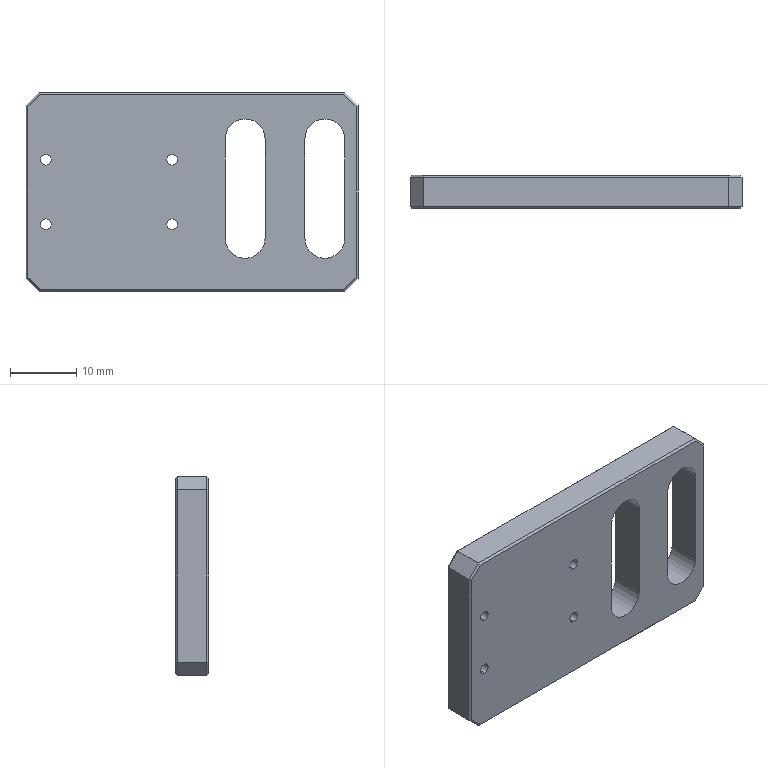Part | SolidWorks | features ICE 3, Chamfer 2, HoleWzd 2, CornerTrim 1, FlatPattern 1, SMBaseFlange 1, SheetMetal 1 | 1 solid | 44 faces | box 50 x 5 x 30 mm | volume 6223 mm3 | plane 30 | cylinder 14 | commonest cylinder face diameters 1.6 x8 6 x6
STEP:
#1=CARTESIAN_POINT('',(40.,0.,11.));
#2=VERTEX_POINT('',#1);
#3=CARTESIAN_POINT('',(43.,0.,8.));
#4=VERTEX_POINT('',#3);
#5=CARTESIAN_POINT('',(40.,0.,8.));
#6=DIRECTION('',(0.,1.,0.));
#7=DIRECTION('',(0.,0.,1.));
#8=AXIS2_PLACEMENT_3D('',#5,#6,#7);
#9=CIRCLE('',#8,3.);
#10=EDGE_CURVE('',#2,#4,#9,.T.);
#11=ORIENTED_EDGE('',*,*,#10,.F.);
#12=CARTESIAN_POINT('',(40.,5.,11.));
#13=VERTEX_POINT('',#12);
#14=CARTESIAN_POINT('',(40.,0.,11.));
#15=DIRECTION('',(0.,1.,0.));
#16=VECTOR('',#15,1000.);
#17=LINE('',#14,#16);
#18=EDGE_CURVE('',#2,#13,#17,.T.);
#19=ORIENTED_EDGE('',*,*,#18,.T.);
#20=CARTESIAN_POINT('',(43.,5.,8.));
#21=VERTEX_POINT('',#20);
#22=CARTESIAN_POINT('',(40.,5.,8.));
#23=DIRECTION('',(0.,1.,0.));
#24=DIRECTION('',(0.,0.,1.));
#25=AXIS2_PLACEMENT_3D('',#22,#23,#24);
#26=CIRCLE('',#25,3.);
#27=EDGE_CURVE('',#13,#21,#26,.T.);
#28=ORIENTED_EDGE('',*,*,#27,.T.);
#29=CARTESIAN_POINT('',(43.,0.,8.));
#30=DIRECTION('',(0.,1.,0.));
#31=VECTOR('',#30,1000.);
#32=LINE('',#29,#31);
#33=EDGE_CURVE('',#4,#21,#32,.T.);
#34=ORIENTED_EDGE('',*,*,#33,.F.);
#35=EDGE_LOOP('',(#11,#19,#28,#34));
#36=FACE_OUTER_BOUND('',#35,.T.);
#37=CARTESIAN_POINT('',(40.,0.,8.));
#38=DIRECTION('',(0.,1.,0.));
#39=DIRECTION('',(0.,0.,1.));
#40=AXIS2_PLACEMENT_3D('',#37,#38,#39);
#41=CYLINDRICAL_SURFACE('',#40,3.);
#42=ADVANCED_FACE('',(#36),#41,.F.);
#43=CARTESIAN_POINT('',(28.,0.,11.));
#44=VERTEX_POINT('',#43);
#45=CARTESIAN_POINT('',(31.,0.,8.));
#46=VERTEX_POINT('',#45);
#47=CARTESIAN_POINT('',(28.,0.,8.));
#48=DIRECTION('',(0.,1.,0.));
#49=DIRECTION('',(0.,0.,1.));
#50=AXIS2_PLACEMENT_3D('',#47,#48,#49);
#51=CIRCLE('',#50,3.);
#52=EDGE_CURVE('',#44,#46,#51,.T.);
#53=ORIENTED_EDGE('',*,*,#52,.F.);
#54=CARTESIAN_POINT('',(28.,5.,11.));
#55=VERTEX_POINT('',#54);
#56=CARTESIAN_POINT('',(28.,0.,11.));
#57=DIRECTION('',(0.,1.,0.));
#58=VECTOR('',#57,1000.);
#59=LINE('',#56,#58);
#60=EDGE_CURVE('',#44,#55,#59,.T.);
#61=ORIENTED_EDGE('',*,*,#60,.T.);
#62=CARTESIAN_POINT('',(31.,5.,8.));
#63=VERTEX_POINT('',#62);
#64=CARTESIAN_POINT('',(28.,5.,8.));
#65=DIRECTION('',(0.,1.,0.));
#66=DIRECTION('',(0.,0.,1.));
#67=AXIS2_PLACEMENT_3D('',#64,#65,#66);
#68=CIRCLE('',#67,3.);
#69=EDGE_CURVE('',#55,#63,#68,.T.);
#70=ORIENTED_EDGE('',*,*,#69,.T.);
#71=CARTESIAN_POINT('',(31.,0.,8.));
#72=DIRECTION('',(0.,1.,0.));
#73=VECTOR('',#72,1000.);
#74=LINE('',#71,#73);
#75=EDGE_CURVE('',#46,#63,#74,.T.);
#76=ORIENTED_EDGE('',*,*,#75,.F.);
#77=EDGE_LOOP('',(#53,#61,#70,#76));
#78=FACE_OUTER_BOUND('',#77,.T.);
#79=CARTESIAN_POINT('',(28.,0.,8.));
#80=DIRECTION('',(0.,1.,0.));
#81=DIRECTION('',(0.,0.,1.));
#82=AXIS2_PLACEMENT_3D('',#79,#80,#81);
#83=CYLINDRICAL_SURFACE('',#82,3.);
#84=ADVANCED_FACE('',(#78),#83,.F.);
#85=CARTESIAN_POINT('',(17.,0.,-5.65));
#86=VERTEX_POINT('',#85);
#87=CARTESIAN_POINT('',(17.,0.,-4.05));
#88=VERTEX_POINT('',#87);
#89=CARTESIAN_POINT('',(17.,0.,-4.85));
#90=DIRECTION('',(0.,1.,0.));
#91=DIRECTION('',(0.,0.,1.));
#92=AXIS2_PLACEMENT_3D('',#89,#90,#91);
#93=CIRCLE('',#92,0.8);
#94=EDGE_CURVE('',#86,#88,#93,.T.);
#95=ORIENTED_EDGE('',*,*,#94,.F.);
#96=CARTESIAN_POINT('',(17.,5.,-5.65));
#97=VERTEX_POINT('',#96);
#98=CARTESIAN_POINT('',(17.,5.,-5.65));
#99=DIRECTION('',(0.,1.,0.));
#100=VECTOR('',#99,1000.);
#101=LINE('',#98,#100);
#102=EDGE_CURVE('',#86,#97,#101,.T.);
#103=ORIENTED_EDGE('',*,*,#102,.T.);
#104=CARTESIAN_POINT('',(17.,5.,-4.05));
#105=VERTEX_POINT('',#104);
#106=CARTESIAN_POINT('',(17.,5.,-4.85));
#107=DIRECTION('',(0.,1.,0.));
#108=DIRECTION('',(0.,0.,1.));
#109=AXIS2_PLACEMENT_3D('',#106,#107,#108);
#110=CIRCLE('',#109,0.8);
#111=EDGE_CURVE('',#97,#105,#110,.T.);
#112=ORIENTED_EDGE('',*,*,#111,.T.);
#113=CARTESIAN_POINT('',(17.,5.,-4.05));
#114=DIRECTION('',(0.,1.,0.));
#115=VECTOR('',#114,1000.);
#116=LINE('',#113,#115);
#117=EDGE_CURVE('',#88,#105,#116,.T.);
#118=ORIENTED_EDGE('',*,*,#117,.F.);
#119=EDGE_LOOP('',(#95,#103,#112,#118));
#120=FACE_OUTER_BOUND('',#119,.T.);
#121=CARTESIAN_POINT('',(17.,5.,-4.85));
#122=DIRECTION('',(0.,1.,0.));
#123=DIRECTION('',(0.,0.,1.));
#124=AXIS2_PLACEMENT_3D('',#121,#122,#123);
#125=CYLINDRICAL_SURFACE('',#124,0.8);
#126=ADVANCED_FACE('',(#120),#125,.F.);
#127=CARTESIAN_POINT('',(-2.,0.,4.05));
#128=VERTEX_POINT('',#127);
#129=CARTESIAN_POINT('',(-2.,0.,5.65));
#130=VERTEX_POINT('',#129);
#131=CARTESIAN_POINT('',(-2.,0.,4.85));
#132=DIRECTION('',(0.,1.,0.));
#133=DIRECTION('',(0.,0.,1.));
#134=AXIS2_PLACEMENT_3D('',#131,#132,#133);
#135=CIRCLE('',#134,0.8);
#136=EDGE_CURVE('',#128,#130,#135,.T.);
#137=ORIENTED_EDGE('',*,*,#136,.F.);
#138=CARTESIAN_POINT('',(-2.,5.,4.05));
#139=VERTEX_POINT('',#138);
#140=CARTESIAN_POINT('',(-2.,5.,4.05));
#141=DIRECTION('',(0.,1.,0.));
#142=VECTOR('',#141,1000.);
#143=LINE('',#140,#142);
#144=EDGE_CURVE('',#128,#139,#143,.T.);
#145=ORIENTED_EDGE('',*,*,#144,.T.);
#146=CARTESIAN_POINT('',(-2.,5.,5.65));
#147=VERTEX_POINT('',#146);
#148=CARTESIAN_POINT('',(-2.,5.,4.85));
#149=DIRECTION('',(0.,1.,0.));
#150=DIRECTION('',(0.,0.,1.));
#151=AXIS2_PLACEMENT_3D('',#148,#149,#150);
#152=CIRCLE('',#151,0.8);
#153=EDGE_CURVE('',#139,#147,#152,.T.);
#154=ORIENTED_EDGE('',*,*,#153,.T.);
#155=CARTESIAN_POINT('',(-2.,5.,5.65));
#156=DIRECTION('',(0.,1.,0.));
#157=VECTOR('',#156,1000.);
#158=LINE('',#155,#157);
#159=EDGE_CURVE('',#130,#147,#158,.T.);
#160=ORIENTED_EDGE('',*,*,#159,.F.);
#161=EDGE_LOOP('',(#137,#145,#154,#160));
#162=FACE_OUTER_BOUND('',#161,.T.);
#163=CARTESIAN_POINT('',(-2.,5.,4.85));
#164=DIRECTION('',(0.,1.,0.));
#165=DIRECTION('',(0.,0.,1.));
#166=AXIS2_PLACEMENT_3D('',#163,#164,#165);
#167=CYLINDRICAL_SURFACE('',#166,0.8);
#168=ADVANCED_FACE('',(#162),#167,.F.);
#169=CARTESIAN_POINT('',(-2.,0.,-5.65));
#170=VERTEX_POINT('',#169);
#171=CARTESIAN_POINT('',(-2.,0.,-4.05));
#172=VERTEX_POINT('',#171);
#173=CARTESIAN_POINT('',(-2.,0.,-4.85));
#174=DIRECTION('',(0.,1.,0.));
#175=DIRECTION('',(0.,0.,1.));
#176=AXIS2_PLACEMENT_3D('',#173,#174,#175);
#177=CIRCLE('',#176,0.8);
#178=EDGE_CURVE('',#170,#172,#177,.T.);
#179=ORIENTED_EDGE('',*,*,#178,.F.);
#180=CARTESIAN_POINT('',(-2.,5.,-5.65));
#181=VERTEX_POINT('',#180);
#182=CARTESIAN_POINT('',(-2.,5.,-5.65));
#183=DIRECTION('',(0.,1.,0.));
#184=VECTOR('',#183,1000.);
#185=LINE('',#182,#184);
#186=EDGE_CURVE('',#170,#181,#185,.T.);
#187=ORIENTED_EDGE('',*,*,#186,.T.);
#188=CARTESIAN_POINT('',(-2.,5.,-4.05));
#189=VERTEX_POINT('',#188);
#190=CARTESIAN_POINT('',(-2.,5.,-4.85));
#191=DIRECTION('',(0.,1.,0.));
#192=DIRECTION('',(0.,0.,1.));
#193=AXIS2_PLACEMENT_3D('',#190,#191,#192);
#194=CIRCLE('',#193,0.8);
#195=EDGE_CURVE('',#181,#189,#194,.T.);
#196=ORIENTED_EDGE('',*,*,#195,.T.);
#197=CARTESIAN_POINT('',(-2.,5.,-4.05));
#198=DIRECTION('',(0.,1.,0.));
#199=VECTOR('',#198,1000.);
#200=LINE('',#197,#199);
#201=EDGE_CURVE('',#172,#189,#200,.T.);
#202=ORIENTED_EDGE('',*,*,#201,.F.);
#203=EDGE_LOOP('',(#179,#187,#196,#202));
#204=FACE_OUTER_BOUND('',#203,.T.);
#205=CARTESIAN_POINT('',(-2.,5.,-4.85));
#206=DIRECTION('',(0.,1.,0.));
#207=DIRECTION('',(0.,0.,1.));
#208=AXIS2_PLACEMENT_3D('',#205,#206,#207);
#209=CYLINDRICAL_SURFACE('',#208,0.8);
#210=ADVANCED_FACE('',(#204),#209,.F.);
#211=CARTESIAN_POINT('',(17.,0.,4.05));
#212=VERTEX_POINT('',#211);
#213=CARTESIAN_POINT('',(17.,0.,5.65));
#214=VERTEX_POINT('',#213);
#215=CARTESIAN_POINT('',(17.,0.,4.85));
#216=DIRECTION('',(0.,1.,0.));
#217=DIRECTION('',(0.,0.,1.));
#218=AXIS2_PLACEMENT_3D('',#215,#216,#217);
#219=CIRCLE('',#218,0.8);
#220=EDGE_CURVE('',#212,#214,#219,.T.);
#221=ORIENTED_EDGE('',*,*,#220,.F.);
#222=CARTESIAN_POINT('',(17.,5.,4.05));
#223=VERTEX_POINT('',#222);
#224=CARTESIAN_POINT('',(17.,5.,4.05));
#225=DIRECTION('',(0.,1.,0.));
#226=VECTOR('',#225,1000.);
#227=LINE('',#224,#226);
#228=EDGE_CURVE('',#212,#223,#227,.T.);
#229=ORIENTED_EDGE('',*,*,#228,.T.);
#230=CARTESIAN_POINT('',(17.,5.,5.65));
#231=VERTEX_POINT('',#230);
#232=CARTESIAN_POINT('',(17.,5.,4.85));
#233=DIRECTION('',(0.,1.,0.));
#234=DIRECTION('',(0.,0.,1.));
#235=AXIS2_PLACEMENT_3D('',#232,#233,#234);
#236=CIRCLE('',#235,0.8);
#237=EDGE_CURVE('',#223,#231,#236,.T.);
#238=ORIENTED_EDGE('',*,*,#237,.T.);
#239=CARTESIAN_POINT('',(17.,5.,5.65));
#240=DIRECTION('',(0.,1.,0.));
#241=VECTOR('',#240,1000.);
#242=LINE('',#239,#241);
#243=EDGE_CURVE('',#214,#231,#242,.T.);
#244=ORIENTED_EDGE('',*,*,#243,.F.);
#245=EDGE_LOOP('',(#221,#229,#238,#244));
#246=FACE_OUTER_BOUND('',#245,.T.);
#247=CARTESIAN_POINT('',(17.,5.,4.85));
#248=DIRECTION('',(0.,1.,0.));
#249=DIRECTION('',(0.,0.,1.));
#250=AXIS2_PLACEMENT_3D('',#247,#248,#249);
#251=CYLINDRICAL_SURFACE('',#250,0.8);
#252=ADVANCED_FACE('',(#246),#251,.F.);
#253=CARTESIAN_POINT('',(43.,4.7,-15.));
#254=VERTEX_POINT('',#253);
#255=CARTESIAN_POINT('',(43.,0.3,-15.));
#256=VERTEX_POINT('',#255);
#257=CARTESIAN_POINT('',(43.,5.5,-15.));
#258=DIRECTION('',(0.,-1.,0.));
#259=VECTOR('',#258,1000.);
#260=LINE('',#257,#259);
#261=EDGE_CURVE('',#254,#256,#260,.T.);
#262=ORIENTED_EDGE('',*,*,#261,.T.);
#263=CARTESIAN_POINT('',(-3.,0.3,-15.));
#264=VERTEX_POINT('',#263);
#265=CARTESIAN_POINT('',(-40.,0.3,-15.));
#266=DIRECTION('',(-1.,0.,0.));
#267=VECTOR('',#266,1000.);
#268=LINE('',#265,#267);
#269=EDGE_CURVE('',#256,#264,#268,.T.);
#270=ORIENTED_EDGE('',*,*,#269,.T.);
#271=CARTESIAN_POINT('',(-3.,4.7,-15.));
#272=VERTEX_POINT('',#271);
#273=CARTESIAN_POINT('',(-3.,5.,-15.));
#274=DIRECTION('',(0.,1.,0.));
#275=VECTOR('',#274,1000.);
#276=LINE('',#273,#275);
#277=EDGE_CURVE('',#264,#272,#276,.T.);
#278=ORIENTED_EDGE('',*,*,#277,.T.);
#279=CARTESIAN_POINT('',(43.,4.7,-15.));
#280=DIRECTION('',(1.,0.,0.));
#281=VECTOR('',#280,1000.);
#282=LINE('',#279,#281);
#283=EDGE_CURVE('',#272,#254,#282,.T.);
#284=ORIENTED_EDGE('',*,*,#283,.T.);
#285=EDGE_LOOP('',(#262,#270,#278,#284));
#286=FACE_OUTER_BOUND('',#285,.T.);
#287=CARTESIAN_POINT('',(-40.,5.5,-15.));
#288=DIRECTION('',(0.,0.,-1.));
#289=DIRECTION('',(-1.,0.,0.));
#290=AXIS2_PLACEMENT_3D('',#287,#288,#289);
#291=PLANE('',#290);
#292=ADVANCED_FACE('',(#286),#291,.T.);
#293=CARTESIAN_POINT('',(43.,0.,-7.));
#294=VERTEX_POINT('',#293);
#295=CARTESIAN_POINT('',(37.,0.,-7.));
#296=VERTEX_POINT('',#295);
#297=CARTESIAN_POINT('',(40.,0.,-7.));
#298=DIRECTION('',(0.,1.,0.));
#299=DIRECTION('',(0.,0.,1.));
#300=AXIS2_PLACEMENT_3D('',#297,#298,#299);
#301=CIRCLE('',#300,3.);
#302=EDGE_CURVE('',#294,#296,#301,.T.);
#303=ORIENTED_EDGE('',*,*,#302,.T.);
#304=CARTESIAN_POINT('',(37.,0.,8.));
#305=VERTEX_POINT('',#304);
#306=CARTESIAN_POINT('',(37.,0.,-7.));
#307=DIRECTION('',(0.,0.,1.));
#308=VECTOR('',#307,1000.);
#309=LINE('',#306,#308);
#310=EDGE_CURVE('',#296,#305,#309,.T.);
#311=ORIENTED_EDGE('',*,*,#310,.T.);
#312=CARTESIAN_POINT('',(40.,0.,8.));
#313=DIRECTION('',(0.,1.,0.));
#314=DIRECTION('',(0.,0.,1.));
#315=AXIS2_PLACEMENT_3D('',#312,#313,#314);
#316=CIRCLE('',#315,3.);
#317=EDGE_CURVE('',#305,#2,#316,.T.);
#318=ORIENTED_EDGE('',*,*,#317,.T.);
#319=ORIENTED_EDGE('',*,*,#10,.T.);
#320=CARTESIAN_POINT('',(43.,0.,-7.));
#321=DIRECTION('',(0.,0.,-1.));
#322=VECTOR('',#321,1000.);
#323=LINE('',#320,#322);
#324=EDGE_CURVE('',#4,#294,#323,.T.);
#325=ORIENTED_EDGE('',*,*,#324,.T.);
#326=EDGE_LOOP('',(#303,#311,#318,#319,#325));
#327=FACE_BOUND('',#326,.T.);
#328=CARTESIAN_POINT('',(31.,0.,-7.));
#329=VERTEX_POINT('',#328);
#330=CARTESIAN_POINT('',(25.,0.,-7.));
#331=VERTEX_POINT('',#330);
#332=CARTESIAN_POINT('',(28.,0.,-7.));
#333=DIRECTION('',(0.,1.,0.));
#334=DIRECTION('',(0.,0.,1.));
#335=AXIS2_PLACEMENT_3D('',#332,#333,#334);
#336=CIRCLE('',#335,3.);
#337=EDGE_CURVE('',#329,#331,#336,.T.);
#338=ORIENTED_EDGE('',*,*,#337,.T.);
#339=CARTESIAN_POINT('',(25.,0.,8.));
#340=VERTEX_POINT('',#339);
#341=CARTESIAN_POINT('',(25.,0.,-7.));
#342=DIRECTION('',(0.,0.,1.));
#343=VECTOR('',#342,1000.);
#344=LINE('',#341,#343);
#345=EDGE_CURVE('',#331,#340,#344,.T.);
#346=ORIENTED_EDGE('',*,*,#345,.T.);
#347=CARTESIAN_POINT('',(28.,0.,8.));
#348=DIRECTION('',(0.,1.,0.));
#349=DIRECTION('',(0.,0.,1.));
#350=AXIS2_PLACEMENT_3D('',#347,#348,#349);
#351=CIRCLE('',#350,3.);
#352=EDGE_CURVE('',#340,#44,#351,.T.);
#353=ORIENTED_EDGE('',*,*,#352,.T.);
#354=ORIENTED_EDGE('',*,*,#52,.T.);
#355=CARTESIAN_POINT('',(31.,0.,-7.));
#356=DIRECTION('',(0.,0.,-1.));
#357=VECTOR('',#356,1000.);
#358=LINE('',#355,#357);
#359=EDGE_CURVE('',#46,#329,#358,.T.);
#360=ORIENTED_EDGE('',*,*,#359,.T.);
#361=EDGE_LOOP('',(#338,#346,#353,#354,#360));
#362=FACE_BOUND('',#361,.T.);
#363=CARTESIAN_POINT('',(-4.7,0.,12.876));
#364=VERTEX_POINT('',#363);
#365=CARTESIAN_POINT('',(-4.7,0.,-12.876));
#366=VERTEX_POINT('',#365);
#367=CARTESIAN_POINT('',(-4.7,0.,-13.));
#368=DIRECTION('',(0.,0.,-1.));
#369=VECTOR('',#368,1000.);
#370=LINE('',#367,#369);
#371=EDGE_CURVE('',#364,#366,#370,.T.);
#372=ORIENTED_EDGE('',*,*,#371,.T.);
#373=CARTESIAN_POINT('',(-2.876,0.,-14.7));
#374=VERTEX_POINT('',#373);
#375=CARTESIAN_POINT('',(-38.788,0.,21.212));
#376=DIRECTION('',(0.7071,0.,-0.7071));
#377=VECTOR('',#376,1000.);
#378=LINE('',#375,#377);
#379=EDGE_CURVE('',#366,#374,#378,.T.);
#380=ORIENTED_EDGE('',*,*,#379,.T.);
#381=CARTESIAN_POINT('',(42.876,0.,-14.7));
#382=VERTEX_POINT('',#381);
#383=CARTESIAN_POINT('',(-45.,0.,-14.7));
#384=DIRECTION('',(1.,0.,0.));
#385=VECTOR('',#384,1000.);
#386=LINE('',#383,#385);
#387=EDGE_CURVE('',#374,#382,#386,.T.);
#388=ORIENTED_EDGE('',*,*,#387,.T.);
#389=CARTESIAN_POINT('',(44.7,0.,-12.876));
#390=VERTEX_POINT('',#389);
#391=CARTESIAN_POINT('',(13.788,0.,-43.788));
#392=DIRECTION('',(0.7071,0.,0.7071));
#393=VECTOR('',#392,1000.);
#394=LINE('',#391,#393);
#395=EDGE_CURVE('',#382,#390,#394,.T.);
#396=ORIENTED_EDGE('',*,*,#395,.T.);
#397=CARTESIAN_POINT('',(44.7,0.,12.876));
#398=VERTEX_POINT('',#397);
#399=CARTESIAN_POINT('',(44.7,0.,15.));
#400=DIRECTION('',(0.,0.,1.));
#401=VECTOR('',#400,1000.);
#402=LINE('',#399,#401);
#403=EDGE_CURVE('',#390,#398,#402,.T.);
#404=ORIENTED_EDGE('',*,*,#403,.T.);
#405=CARTESIAN_POINT('',(42.876,0.,14.7));
#406=VERTEX_POINT('',#405);
#407=CARTESIAN_POINT('',(-1.212,0.,58.788));
#408=DIRECTION('',(-0.7071,0.,0.7071));
#409=VECTOR('',#408,1000.);
#410=LINE('',#407,#409);
#411=EDGE_CURVE('',#398,#406,#410,.T.);
#412=ORIENTED_EDGE('',*,*,#411,.T.);
#413=CARTESIAN_POINT('',(-2.876,0.,14.7));
#414=VERTEX_POINT('',#413);
#415=CARTESIAN_POINT('',(-45.,0.,14.7));
#416=DIRECTION('',(-1.,0.,0.));
#417=VECTOR('',#416,1000.);
#418=LINE('',#415,#417);
#419=EDGE_CURVE('',#406,#414,#418,.T.);
#420=ORIENTED_EDGE('',*,*,#419,.T.);
#421=CARTESIAN_POINT('',(-23.788,0.,-6.212));
#422=DIRECTION('',(-0.7071,0.,-0.7071));
#423=VECTOR('',#422,1000.);
#424=LINE('',#421,#423);
#425=EDGE_CURVE('',#414,#364,#424,.T.);
#426=ORIENTED_EDGE('',*,*,#425,.T.);
#427=EDGE_LOOP('',(#372,#380,#388,#396,#404,#412,#420,#426));
#428=FACE_OUTER_BOUND('',#427,.T.);
#429=CARTESIAN_POINT('',(17.,0.,-4.85));
#430=DIRECTION('',(0.,1.,0.));
#431=DIRECTION('',(0.,0.,1.));
#432=AXIS2_PLACEMENT_3D('',#429,#430,#431);
#433=CIRCLE('',#432,0.8);
#434=EDGE_CURVE('',#88,#86,#433,.T.);
#435=ORIENTED_EDGE('',*,*,#434,.T.);
#436=ORIENTED_EDGE('',*,*,#94,.T.);
#437=EDGE_LOOP('',(#435,#436));
#438=FACE_BOUND('',#437,.T.);
#439=CARTESIAN_POINT('',(-2.,0.,4.85));
#440=DIRECTION('',(0.,1.,0.));
#441=DIRECTION('',(0.,0.,1.));
#442=AXIS2_PLACEMENT_3D('',#439,#440,#441);
#443=CIRCLE('',#442,0.8);
#444=EDGE_CURVE('',#130,#128,#443,.T.);
#445=ORIENTED_EDGE('',*,*,#444,.T.);
#446=ORIENTED_EDGE('',*,*,#136,.T.);
#447=EDGE_LOOP('',(#445,#446));
#448=FACE_BOUND('',#447,.T.);
#449=CARTESIAN_POINT('',(-2.,0.,-4.85));
#450=DIRECTION('',(0.,1.,0.));
#451=DIRECTION('',(0.,0.,1.));
#452=AXIS2_PLACEMENT_3D('',#449,#450,#451);
#453=CIRCLE('',#452,0.8);
#454=EDGE_CURVE('',#172,#170,#453,.T.);
#455=ORIENTED_EDGE('',*,*,#454,.T.);
#456=ORIENTED_EDGE('',*,*,#178,.T.);
#457=EDGE_LOOP('',(#455,#456));
#458=FACE_BOUND('',#457,.T.);
#459=CARTESIAN_POINT('',(17.,0.,4.85));
#460=DIRECTION('',(0.,1.,0.));
#461=DIRECTION('',(0.,0.,1.));
#462=AXIS2_PLACEMENT_3D('',#459,#460,#461);
#463=CIRCLE('',#462,0.8);
#464=EDGE_CURVE('',#214,#212,#463,.T.);
#465=ORIENTED_EDGE('',*,*,#464,.T.);
#466=ORIENTED_EDGE('',*,*,#220,.T.);
#467=EDGE_LOOP('',(#465,#466));
#468=FACE_BOUND('',#467,.T.);
#469=CARTESIAN_POINT('',(-45.,0.,15.));
#470=DIRECTION('',(0.,-1.,0.));
#471=DIRECTION('',(0.,0.,-1.));
#472=AXIS2_PLACEMENT_3D('',#469,#470,#471);
#473=PLANE('',#472);
#474=ADVANCED_FACE('',(#327,#362,#428,#438,#448,#458,#468),#473,.T.);
#475=CARTESIAN_POINT('',(45.,4.7,13.));
#476=VERTEX_POINT('',#475);
#477=CARTESIAN_POINT('',(45.,0.3,13.));
#478=VERTEX_POINT('',#477);
#479=CARTESIAN_POINT('',(45.,5.,13.));
#480=DIRECTION('',(0.,-1.,0.));
#481=VECTOR('',#480,1000.);
#482=LINE('',#479,#481);
#483=EDGE_CURVE('',#476,#478,#482,.T.);
#484=ORIENTED_EDGE('',*,*,#483,.T.);
#485=CARTESIAN_POINT('',(45.,0.3,-13.));
#486=VERTEX_POINT('',#485);
#487=CARTESIAN_POINT('',(45.,0.3,15.));
#488=DIRECTION('',(0.,0.,-1.));
#489=VECTOR('',#488,1000.);
#490=LINE('',#487,#489);
#491=EDGE_CURVE('',#478,#486,#490,.T.);
#492=ORIENTED_EDGE('',*,*,#491,.T.);
#493=CARTESIAN_POINT('',(45.,4.7,-13.));
#494=VERTEX_POINT('',#493);
#495=CARTESIAN_POINT('',(45.,5.,-13.));
#496=DIRECTION('',(0.,1.,0.));
#497=VECTOR('',#496,1000.);
#498=LINE('',#495,#497);
#499=EDGE_CURVE('',#486,#494,#498,.T.);
#500=ORIENTED_EDGE('',*,*,#499,.T.);
#501=CARTESIAN_POINT('',(45.,4.7,13.));
#502=DIRECTION('',(0.,0.,1.));
#503=VECTOR('',#502,1000.);
#504=LINE('',#501,#503);
#505=EDGE_CURVE('',#494,#476,#504,.T.);
#506=ORIENTED_EDGE('',*,*,#505,.T.);
#507=EDGE_LOOP('',(#484,#492,#500,#506));
#508=FACE_OUTER_BOUND('',#507,.T.);
#509=CARTESIAN_POINT('',(45.,5.,15.));
#510=DIRECTION('',(1.,0.,0.));
#511=DIRECTION('',(0.,0.,-1.));
#512=AXIS2_PLACEMENT_3D('',#509,#510,#511);
#513=PLANE('',#512);
#514=ADVANCED_FACE('',(#508),#513,.T.);
#515=CARTESIAN_POINT('',(44.7,5.,12.876));
#516=VERTEX_POINT('',#515);
#517=CARTESIAN_POINT('',(44.7,5.,-12.876));
#518=VERTEX_POINT('',#517);
#519=CARTESIAN_POINT('',(44.7,5.,-13.));
#520=DIRECTION('',(0.,0.,-1.));
#521=VECTOR('',#520,1000.);
#522=LINE('',#519,#521);
#523=EDGE_CURVE('',#516,#518,#522,.T.);
#524=ORIENTED_EDGE('',*,*,#523,.T.);
#525=CARTESIAN_POINT('',(42.876,5.,-14.7));
#526=VERTEX_POINT('',#525);
#527=CARTESIAN_POINT('',(42.788,5.,-14.788));
#528=DIRECTION('',(-0.7071,0.,-0.7071));
#529=VECTOR('',#528,1000.);
#530=LINE('',#527,#529);
#531=EDGE_CURVE('',#518,#526,#530,.T.);
#532=ORIENTED_EDGE('',*,*,#531,.T.);
#533=CARTESIAN_POINT('',(-2.876,5.,-14.7));
#534=VERTEX_POINT('',#533);
#535=CARTESIAN_POINT('',(-3.,5.,-14.7));
#536=DIRECTION('',(-1.,0.,0.));
#537=VECTOR('',#536,1000.);
#538=LINE('',#535,#537);
#539=EDGE_CURVE('',#526,#534,#538,.T.);
#540=ORIENTED_EDGE('',*,*,#539,.T.);
#541=CARTESIAN_POINT('',(-4.7,5.,-12.876));
#542=VERTEX_POINT('',#541);
#543=CARTESIAN_POINT('',(-4.788,5.,-12.788));
#544=DIRECTION('',(-0.7071,0.,0.7071));
#545=VECTOR('',#544,1000.);
#546=LINE('',#543,#545);
#547=EDGE_CURVE('',#534,#542,#546,.T.);
#548=ORIENTED_EDGE('',*,*,#547,.T.);
#549=CARTESIAN_POINT('',(-4.7,5.,12.876));
#550=VERTEX_POINT('',#549);
#551=CARTESIAN_POINT('',(-4.7,5.,15.));
#552=DIRECTION('',(0.,0.,1.));
#553=VECTOR('',#552,1000.);
#554=LINE('',#551,#553);
#555=EDGE_CURVE('',#542,#550,#554,.T.);
#556=ORIENTED_EDGE('',*,*,#555,.T.);
#557=CARTESIAN_POINT('',(-2.876,5.,14.7));
#558=VERTEX_POINT('',#557);
#559=CARTESIAN_POINT('',(-2.788,5.,14.788));
#560=DIRECTION('',(0.7071,0.,0.7071));
#561=VECTOR('',#560,1000.);
#562=LINE('',#559,#561);
#563=EDGE_CURVE('',#550,#558,#562,.T.);
#564=ORIENTED_EDGE('',*,*,#563,.T.);
#565=CARTESIAN_POINT('',(42.876,5.,14.7));
#566=VERTEX_POINT('',#565);
#567=CARTESIAN_POINT('',(43.,5.,14.7));
#568=DIRECTION('',(1.,0.,0.));
#569=VECTOR('',#568,1000.);
#570=LINE('',#567,#569);
#571=EDGE_CURVE('',#558,#566,#570,.T.);
#572=ORIENTED_EDGE('',*,*,#571,.T.);
#573=CARTESIAN_POINT('',(44.788,5.,12.788));
#574=DIRECTION('',(0.7071,0.,-0.7071));
#575=VECTOR('',#574,1000.);
#576=LINE('',#573,#575);
#577=EDGE_CURVE('',#566,#516,#576,.T.);
#578=ORIENTED_EDGE('',*,*,#577,.T.);
#579=EDGE_LOOP('',(#524,#532,#540,#548,#556,#564,#572,#578));
#580=FACE_OUTER_BOUND('',#579,.T.);
#581=CARTESIAN_POINT('',(37.,5.,-7.));
#582=VERTEX_POINT('',#581);
#583=CARTESIAN_POINT('',(37.,5.,8.));
#584=VERTEX_POINT('',#583);
#585=CARTESIAN_POINT('',(37.,5.,-7.));
#586=DIRECTION('',(0.,0.,1.));
#587=VECTOR('',#586,1000.);
#588=LINE('',#585,#587);
#589=EDGE_CURVE('',#582,#584,#588,.T.);
#590=ORIENTED_EDGE('',*,*,#589,.F.);
#591=CARTESIAN_POINT('',(43.,5.,-7.));
#592=VERTEX_POINT('',#591);
#593=CARTESIAN_POINT('',(40.,5.,-7.));
#594=DIRECTION('',(0.,1.,0.));
#595=DIRECTION('',(0.,0.,1.));
#596=AXIS2_PLACEMENT_3D('',#593,#594,#595);
#597=CIRCLE('',#596,3.);
#598=EDGE_CURVE('',#592,#582,#597,.T.);
#599=ORIENTED_EDGE('',*,*,#598,.F.);
#600=CARTESIAN_POINT('',(43.,5.,-7.));
#601=DIRECTION('',(0.,0.,-1.));
#602=VECTOR('',#601,1000.);
#603=LINE('',#600,#602);
#604=EDGE_CURVE('',#21,#592,#603,.T.);
#605=ORIENTED_EDGE('',*,*,#604,.F.);
#606=ORIENTED_EDGE('',*,*,#27,.F.);
#607=CARTESIAN_POINT('',(40.,5.,8.));
#608=DIRECTION('',(0.,1.,0.));
#609=DIRECTION('',(0.,0.,1.));
#610=AXIS2_PLACEMENT_3D('',#607,#608,#609);
#611=CIRCLE('',#610,3.);
#612=EDGE_CURVE('',#584,#13,#611,.T.);
#613=ORIENTED_EDGE('',*,*,#612,.F.);
#614=EDGE_LOOP('',(#590,#599,#605,#606,#613));
#615=FACE_BOUND('',#614,.T.);
#616=CARTESIAN_POINT('',(25.,5.,-7.));
#617=VERTEX_POINT('',#616);
#618=CARTESIAN_POINT('',(25.,5.,8.));
#619=VERTEX_POINT('',#618);
#620=CARTESIAN_POINT('',(25.,5.,-7.));
#621=DIRECTION('',(0.,0.,1.));
#622=VECTOR('',#621,1000.);
#623=LINE('',#620,#622);
#624=EDGE_CURVE('',#617,#619,#623,.T.);
#625=ORIENTED_EDGE('',*,*,#624,.F.);
#626=CARTESIAN_POINT('',(31.,5.,-7.));
#627=VERTEX_POINT('',#626);
#628=CARTESIAN_POINT('',(28.,5.,-7.));
#629=DIRECTION('',(0.,1.,0.));
#630=DIRECTION('',(0.,0.,1.));
#631=AXIS2_PLACEMENT_3D('',#628,#629,#630);
#632=CIRCLE('',#631,3.);
#633=EDGE_CURVE('',#627,#617,#632,.T.);
#634=ORIENTED_EDGE('',*,*,#633,.F.);
#635=CARTESIAN_POINT('',(31.,5.,-7.));
#636=DIRECTION('',(0.,0.,-1.));
#637=VECTOR('',#636,1000.);
#638=LINE('',#635,#637);
#639=EDGE_CURVE('',#63,#627,#638,.T.);
#640=ORIENTED_EDGE('',*,*,#639,.F.);
#641=ORIENTED_EDGE('',*,*,#69,.F.);
#642=CARTESIAN_POINT('',(28.,5.,8.));
#643=DIRECTION('',(0.,1.,0.));
#644=DIRECTION('',(0.,0.,1.));
#645=AXIS2_PLACEMENT_3D('',#642,#643,#644);
#646=CIRCLE('',#645,3.);
#647=EDGE_CURVE('',#619,#55,#646,.T.);
#648=ORIENTED_EDGE('',*,*,#647,.F.);
#649=EDGE_LOOP('',(#625,#634,#640,#641,#648));
#650=FACE_BOUND('',#649,.T.);
#651=CARTESIAN_POINT('',(17.,5.,-4.85));
#652=DIRECTION('',(0.,1.,0.));
#653=DIRECTION('',(0.,0.,1.));
#654=AXIS2_PLACEMENT_3D('',#651,#652,#653);
#655=CIRCLE('',#654,0.8);
#656=EDGE_CURVE('',#105,#97,#655,.T.);
#657=ORIENTED_EDGE('',*,*,#656,.F.);
#658=ORIENTED_EDGE('',*,*,#111,.F.);
#659=EDGE_LOOP('',(#657,#658));
#660=FACE_BOUND('',#659,.T.);
#661=CARTESIAN_POINT('',(-2.,5.,4.85));
#662=DIRECTION('',(0.,1.,0.));
#663=DIRECTION('',(0.,0.,1.));
#664=AXIS2_PLACEMENT_3D('',#661,#662,#663);
#665=CIRCLE('',#664,0.8);
#666=EDGE_CURVE('',#147,#139,#665,.T.);
#667=ORIENTED_EDGE('',*,*,#666,.F.);
#668=ORIENTED_EDGE('',*,*,#153,.F.);
#669=EDGE_LOOP('',(#667,#668));
#670=FACE_BOUND('',#669,.T.);
#671=CARTESIAN_POINT('',(-2.,5.,-4.85));
#672=DIRECTION('',(0.,1.,0.));
#673=DIRECTION('',(0.,0.,1.));
#674=AXIS2_PLACEMENT_3D('',#671,#672,#673);
#675=CIRCLE('',#674,0.8);
#676=EDGE_CURVE('',#189,#181,#675,.T.);
#677=ORIENTED_EDGE('',*,*,#676,.F.);
#678=ORIENTED_EDGE('',*,*,#195,.F.);
#679=EDGE_LOOP('',(#677,#678));
#680=FACE_BOUND('',#679,.T.);
#681=CARTESIAN_POINT('',(17.,5.,4.85));
#682=DIRECTION('',(0.,1.,0.));
#683=DIRECTION('',(0.,0.,1.));
#684=AXIS2_PLACEMENT_3D('',#681,#682,#683);
#685=CIRCLE('',#684,0.8);
#686=EDGE_CURVE('',#231,#223,#685,.T.);
#687=ORIENTED_EDGE('',*,*,#686,.F.);
#688=ORIENTED_EDGE('',*,*,#237,.F.);
#689=EDGE_LOOP('',(#687,#688));
#690=FACE_BOUND('',#689,.T.);
#691=CARTESIAN_POINT('',(-45.,5.,15.));
#692=DIRECTION('',(0.,-1.,0.));
#693=DIRECTION('',(0.,0.,-1.));
#694=AXIS2_PLACEMENT_3D('',#691,#692,#693);
#695=PLANE('',#694);
#696=ADVANCED_FACE('',(#580,#615,#650,#660,#670,#680,#690),#695,.F.);
#697=CARTESIAN_POINT('',(-3.,4.7,15.));
#698=VERTEX_POINT('',#697);
#699=CARTESIAN_POINT('',(-3.,0.3,15.));
#700=VERTEX_POINT('',#699);
#701=CARTESIAN_POINT('',(-3.,0.,15.));
#702=DIRECTION('',(0.,-1.,0.));
#703=VECTOR('',#702,1000.);
#704=LINE('',#701,#703);
#705=EDGE_CURVE('',#698,#700,#704,.T.);
#706=ORIENTED_EDGE('',*,*,#705,.T.);
#707=CARTESIAN_POINT('',(43.,0.3,15.));
#708=VERTEX_POINT('',#707);
#709=CARTESIAN_POINT('',(-39.5,0.3,15.));
#710=DIRECTION('',(1.,0.,0.));
#711=VECTOR('',#710,1000.);
#712=LINE('',#709,#711);
#713=EDGE_CURVE('',#700,#708,#712,.T.);
#714=ORIENTED_EDGE('',*,*,#713,.T.);
#715=CARTESIAN_POINT('',(43.,4.7,15.));
#716=VERTEX_POINT('',#715);
#717=CARTESIAN_POINT('',(43.,5.5,15.));
#718=DIRECTION('',(0.,1.,0.));
#719=VECTOR('',#718,1000.);
#720=LINE('',#717,#719);
#721=EDGE_CURVE('',#708,#716,#720,.T.);
#722=ORIENTED_EDGE('',*,*,#721,.T.);
#723=CARTESIAN_POINT('',(-3.,4.7,15.));
#724=DIRECTION('',(-1.,0.,0.));
#725=VECTOR('',#724,1000.);
#726=LINE('',#723,#725);
#727=EDGE_CURVE('',#716,#698,#726,.T.);
#728=ORIENTED_EDGE('',*,*,#727,.T.);
#729=EDGE_LOOP('',(#706,#714,#722,#728));
#730=FACE_OUTER_BOUND('',#729,.T.);
#731=CARTESIAN_POINT('',(-39.5,5.5,15.));
#732=DIRECTION('',(0.,0.,1.));
#733=DIRECTION('',(1.,0.,0.));
#734=AXIS2_PLACEMENT_3D('',#731,#732,#733);
#735=PLANE('',#734);
#736=ADVANCED_FACE('',(#730),#735,.T.);
#737=ORIENTED_EDGE('',*,*,#721,.F.);
#738=CARTESIAN_POINT('',(45.,0.3,13.));
#739=DIRECTION('',(0.7071,0.,-0.7071));
#740=VECTOR('',#739,1000.);
#741=LINE('',#738,#740);
#742=EDGE_CURVE('',#708,#478,#741,.T.);
#743=ORIENTED_EDGE('',*,*,#742,.T.);
#744=ORIENTED_EDGE('',*,*,#483,.F.);
#745=CARTESIAN_POINT('',(43.,4.7,15.));
#746=DIRECTION('',(-0.7071,0.,0.7071));
#747=VECTOR('',#746,1000.);
#748=LINE('',#745,#747);
#749=EDGE_CURVE('',#476,#716,#748,.T.);
#750=ORIENTED_EDGE('',*,*,#749,.T.);
#751=EDGE_LOOP('',(#737,#743,#744,#750));
#752=FACE_OUTER_BOUND('',#751,.T.);
#753=CARTESIAN_POINT('',(45.,5.,13.));
#754=DIRECTION('',(-0.7071,0.,-0.7071));
#755=DIRECTION('',(0.,-1.,0.));
#756=AXIS2_PLACEMENT_3D('',#753,#754,#755);
#757=PLANE('',#756);
#758=ADVANCED_FACE('',(#752),#757,.F.);
#759=ORIENTED_EDGE('',*,*,#499,.F.);
#760=CARTESIAN_POINT('',(43.,0.3,-15.));
#761=DIRECTION('',(-0.7071,0.,-0.7071));
#762=VECTOR('',#761,1000.);
#763=LINE('',#760,#762);
#764=EDGE_CURVE('',#486,#256,#763,.T.);
#765=ORIENTED_EDGE('',*,*,#764,.T.);
#766=ORIENTED_EDGE('',*,*,#261,.F.);
#767=CARTESIAN_POINT('',(45.,4.7,-13.));
#768=DIRECTION('',(0.7071,0.,0.7071));
#769=VECTOR('',#768,1000.);
#770=LINE('',#767,#769);
#771=EDGE_CURVE('',#254,#494,#770,.T.);
#772=ORIENTED_EDGE('',*,*,#771,.T.);
#773=EDGE_LOOP('',(#759,#765,#766,#772));
#774=FACE_OUTER_BOUND('',#773,.T.);
#775=CARTESIAN_POINT('',(43.,5.5,-15.));
#776=DIRECTION('',(-0.7071,0.,0.7071));
#777=DIRECTION('',(0.,-1.,0.));
#778=AXIS2_PLACEMENT_3D('',#775,#776,#777);
#779=PLANE('',#778);
#780=ADVANCED_FACE('',(#774),#779,.F.);
#781=ORIENTED_EDGE('',*,*,#228,.F.);
#782=ORIENTED_EDGE('',*,*,#464,.F.);
#783=ORIENTED_EDGE('',*,*,#243,.T.);
#784=ORIENTED_EDGE('',*,*,#686,.T.);
#785=EDGE_LOOP('',(#781,#782,#783,#784));
#786=FACE_OUTER_BOUND('',#785,.T.);
#787=CARTESIAN_POINT('',(17.,5.,4.85));
#788=DIRECTION('',(0.,1.,0.));
#789=DIRECTION('',(0.,0.,1.));
#790=AXIS2_PLACEMENT_3D('',#787,#788,#789);
#791=CYLINDRICAL_SURFACE('',#790,0.8);
#792=ADVANCED_FACE('',(#786),#791,.F.);
#793=ORIENTED_EDGE('',*,*,#186,.F.);
#794=ORIENTED_EDGE('',*,*,#454,.F.);
#795=ORIENTED_EDGE('',*,*,#201,.T.);
#796=ORIENTED_EDGE('',*,*,#676,.T.);
#797=EDGE_LOOP('',(#793,#794,#795,#796));
#798=FACE_OUTER_BOUND('',#797,.T.);
#799=CARTESIAN_POINT('',(-2.,5.,-4.85));
#800=DIRECTION('',(0.,1.,0.));
#801=DIRECTION('',(0.,0.,1.));
#802=AXIS2_PLACEMENT_3D('',#799,#800,#801);
#803=CYLINDRICAL_SURFACE('',#802,0.8);
#804=ADVANCED_FACE('',(#798),#803,.F.);
#805=ORIENTED_EDGE('',*,*,#144,.F.);
#806=ORIENTED_EDGE('',*,*,#444,.F.);
#807=ORIENTED_EDGE('',*,*,#159,.T.);
#808=ORIENTED_EDGE('',*,*,#666,.T.);
#809=EDGE_LOOP('',(#805,#806,#807,#808));
#810=FACE_OUTER_BOUND('',#809,.T.);
#811=CARTESIAN_POINT('',(-2.,5.,4.85));
#812=DIRECTION('',(0.,1.,0.));
#813=DIRECTION('',(0.,0.,1.));
#814=AXIS2_PLACEMENT_3D('',#811,#812,#813);
#815=CYLINDRICAL_SURFACE('',#814,0.8);
#816=ADVANCED_FACE('',(#810),#815,.F.);
#817=ORIENTED_EDGE('',*,*,#102,.F.);
#818=ORIENTED_EDGE('',*,*,#434,.F.);
#819=ORIENTED_EDGE('',*,*,#117,.T.);
#820=ORIENTED_EDGE('',*,*,#656,.T.);
#821=EDGE_LOOP('',(#817,#818,#819,#820));
#822=FACE_OUTER_BOUND('',#821,.T.);
#823=CARTESIAN_POINT('',(17.,5.,-4.85));
#824=DIRECTION('',(0.,1.,0.));
#825=DIRECTION('',(0.,0.,1.));
#826=AXIS2_PLACEMENT_3D('',#823,#824,#825);
#827=CYLINDRICAL_SURFACE('',#826,0.8);
#828=ADVANCED_FACE('',(#822),#827,.F.);
#829=CARTESIAN_POINT('',(-5.,4.7,-13.));
#830=VERTEX_POINT('',#829);
#831=CARTESIAN_POINT('',(-5.,0.3,-13.));
#832=VERTEX_POINT('',#831);
#833=CARTESIAN_POINT('',(-5.,0.,-13.));
#834=DIRECTION('',(0.,-1.,0.));
#835=VECTOR('',#834,1000.);
#836=LINE('',#833,#835);
#837=EDGE_CURVE('',#830,#832,#836,.T.);
#838=ORIENTED_EDGE('',*,*,#837,.T.);
#839=CARTESIAN_POINT('',(-5.,0.3,13.));
#840=VERTEX_POINT('',#839);
#841=CARTESIAN_POINT('',(-5.,0.3,13.));
#842=DIRECTION('',(0.,0.,1.));
#843=VECTOR('',#842,1000.);
#844=LINE('',#841,#843);
#845=EDGE_CURVE('',#832,#840,#844,.T.);
#846=ORIENTED_EDGE('',*,*,#845,.T.);
#847=CARTESIAN_POINT('',(-5.,4.7,13.));
#848=VERTEX_POINT('',#847);
#849=CARTESIAN_POINT('',(-5.,5.,13.));
#850=DIRECTION('',(0.,1.,0.));
#851=VECTOR('',#850,1000.);
#852=LINE('',#849,#851);
#853=EDGE_CURVE('',#840,#848,#852,.T.);
#854=ORIENTED_EDGE('',*,*,#853,.T.);
#855=CARTESIAN_POINT('',(-5.,4.7,25.052));
#856=DIRECTION('',(0.,0.,-1.));
#857=VECTOR('',#856,1000.);
#858=LINE('',#855,#857);
#859=EDGE_CURVE('',#848,#830,#858,.T.);
#860=ORIENTED_EDGE('',*,*,#859,.T.);
#861=EDGE_LOOP('',(#838,#846,#854,#860));
#862=FACE_OUTER_BOUND('',#861,.T.);
#863=CARTESIAN_POINT('',(-5.,15.,25.052));
#864=DIRECTION('',(1.,0.,0.));
#865=DIRECTION('',(0.,0.,-1.));
#866=AXIS2_PLACEMENT_3D('',#863,#864,#865);
#867=PLANE('',#866);
#868=ADVANCED_FACE('',(#862),#867,.F.);
#869=ORIENTED_EDGE('',*,*,#853,.F.);
#870=CARTESIAN_POINT('',(-5.,0.3,13.));
#871=DIRECTION('',(0.7071,0.,0.7071));
#872=VECTOR('',#871,1000.);
#873=LINE('',#870,#872);
#874=EDGE_CURVE('',#840,#700,#873,.T.);
#875=ORIENTED_EDGE('',*,*,#874,.T.);
#876=ORIENTED_EDGE('',*,*,#705,.F.);
#877=CARTESIAN_POINT('',(-5.,4.7,13.));
#878=DIRECTION('',(-0.7071,0.,-0.7071));
#879=VECTOR('',#878,1000.);
#880=LINE('',#877,#879);
#881=EDGE_CURVE('',#698,#848,#880,.T.);
#882=ORIENTED_EDGE('',*,*,#881,.T.);
#883=EDGE_LOOP('',(#869,#875,#876,#882));
#884=FACE_OUTER_BOUND('',#883,.T.);
#885=CARTESIAN_POINT('',(-5.,15.,13.));
#886=DIRECTION('',(-0.7071,0.,0.7071));
#887=DIRECTION('',(0.,-1.,0.));
#888=AXIS2_PLACEMENT_3D('',#885,#886,#887);
#889=PLANE('',#888);
#890=ADVANCED_FACE('',(#884),#889,.T.);
#891=ORIENTED_EDGE('',*,*,#277,.F.);
#892=CARTESIAN_POINT('',(-5.,0.3,-13.));
#893=DIRECTION('',(-0.7071,0.,0.7071));
#894=VECTOR('',#893,1000.);
#895=LINE('',#892,#894);
#896=EDGE_CURVE('',#264,#832,#895,.T.);
#897=ORIENTED_EDGE('',*,*,#896,.T.);
#898=ORIENTED_EDGE('',*,*,#837,.F.);
#899=CARTESIAN_POINT('',(-3.,4.7,-15.));
#900=DIRECTION('',(0.7071,0.,-0.7071));
#901=VECTOR('',#900,1000.);
#902=LINE('',#899,#901);
#903=EDGE_CURVE('',#830,#272,#902,.T.);
#904=ORIENTED_EDGE('',*,*,#903,.T.);
#905=EDGE_LOOP('',(#891,#897,#898,#904));
#906=FACE_OUTER_BOUND('',#905,.T.);
#907=CARTESIAN_POINT('',(-5.,15.,-13.));
#908=DIRECTION('',(-0.7071,0.,-0.7071));
#909=DIRECTION('',(0.,1.,0.));
#910=AXIS2_PLACEMENT_3D('',#907,#908,#909);
#911=PLANE('',#910);
#912=ADVANCED_FACE('',(#906),#911,.T.);
#913=CARTESIAN_POINT('',(45.381,0.6815,13.158));
#914=DIRECTION('',(-0.6786,-0.6786,-0.2811));
#915=VECTOR('',#914,1000.);
#916=LINE('',#913,#915);
#917=EDGE_CURVE('',#478,#398,#916,.T.);
#918=ORIENTED_EDGE('',*,*,#917,.F.);
#919=ORIENTED_EDGE('',*,*,#742,.F.);
#920=CARTESIAN_POINT('',(47.802,11.893,26.593));
#921=DIRECTION('',(0.2811,0.6786,0.6786));
#922=VECTOR('',#921,1000.);
#923=LINE('',#920,#922);
#924=EDGE_CURVE('',#406,#708,#923,.T.);
#925=ORIENTED_EDGE('',*,*,#924,.F.);
#926=ORIENTED_EDGE('',*,*,#411,.F.);
#927=EDGE_LOOP('',(#918,#919,#925,#926));
#928=FACE_OUTER_BOUND('',#927,.T.);
#929=CARTESIAN_POINT('',(-1.212,0.,58.788));
#930=DIRECTION('',(0.5,-0.7071,0.5));
#931=DIRECTION('',(0.7071,0.,-0.7071));
#932=AXIS2_PLACEMENT_3D('',#929,#930,#931);
#933=PLANE('',#932);
#934=ADVANCED_FACE('',(#928),#933,.T.);
#935=ORIENTED_EDGE('',*,*,#924,.T.);
#936=ORIENTED_EDGE('',*,*,#713,.F.);
#937=CARTESIAN_POINT('',(-6.204,8.035,22.735));
#938=DIRECTION('',(-0.2811,0.6786,0.6786));
#939=VECTOR('',#938,1000.);
#940=LINE('',#937,#939);
#941=EDGE_CURVE('',#414,#700,#940,.T.);
#942=ORIENTED_EDGE('',*,*,#941,.F.);
#943=ORIENTED_EDGE('',*,*,#419,.F.);
#944=EDGE_LOOP('',(#935,#936,#942,#943));
#945=FACE_OUTER_BOUND('',#944,.T.);
#946=CARTESIAN_POINT('',(-45.,0.,14.7));
#947=DIRECTION('',(0.,0.7071,-0.7071));
#948=DIRECTION('',(-1.,0.,0.));
#949=AXIS2_PLACEMENT_3D('',#946,#947,#948);
#950=PLANE('',#949);
#951=ADVANCED_FACE('',(#945),#950,.F.);
#952=ORIENTED_EDGE('',*,*,#917,.T.);
#953=ORIENTED_EDGE('',*,*,#403,.F.);
#954=CARTESIAN_POINT('',(36.361,-8.339,-9.422));
#955=DIRECTION('',(-0.6786,-0.6786,0.2811));
#956=VECTOR('',#955,1000.);
#957=LINE('',#954,#956);
#958=EDGE_CURVE('',#486,#390,#957,.T.);
#959=ORIENTED_EDGE('',*,*,#958,.F.);
#960=ORIENTED_EDGE('',*,*,#491,.F.);
#961=EDGE_LOOP('',(#952,#953,#959,#960));
#962=FACE_OUTER_BOUND('',#961,.T.);
#963=CARTESIAN_POINT('',(45.,0.3,15.));
#964=DIRECTION('',(-0.7071,0.7071,0.));
#965=DIRECTION('',(0.,0.,-1.));
#966=AXIS2_PLACEMENT_3D('',#963,#964,#965);
#967=PLANE('',#966);
#968=ADVANCED_FACE('',(#962),#967,.F.);
#969=ORIENTED_EDGE('',*,*,#941,.T.);
#970=ORIENTED_EDGE('',*,*,#874,.F.);
#971=CARTESIAN_POINT('',(-9.849,5.149,15.009));
#972=DIRECTION('',(-0.6786,0.6786,0.2811));
#973=VECTOR('',#972,1000.);
#974=LINE('',#971,#973);
#975=EDGE_CURVE('',#364,#840,#974,.T.);
#976=ORIENTED_EDGE('',*,*,#975,.F.);
#977=ORIENTED_EDGE('',*,*,#425,.F.);
#978=EDGE_LOOP('',(#969,#970,#976,#977));
#979=FACE_OUTER_BOUND('',#978,.T.);
#980=CARTESIAN_POINT('',(-23.788,0.,-6.212));
#981=DIRECTION('',(0.5,0.7071,-0.5));
#982=DIRECTION('',(-0.7071,0.,-0.7071));
#983=AXIS2_PLACEMENT_3D('',#980,#981,#982);
#984=PLANE('',#983);
#985=ADVANCED_FACE('',(#979),#984,.F.);
#986=ORIENTED_EDGE('',*,*,#958,.T.);
#987=ORIENTED_EDGE('',*,*,#395,.F.);
#988=CARTESIAN_POINT('',(46.126,7.847,-22.547));
#989=DIRECTION('',(-0.2811,-0.6786,0.6786));
#990=VECTOR('',#989,1000.);
#991=LINE('',#988,#990);
#992=EDGE_CURVE('',#256,#382,#991,.T.);
#993=ORIENTED_EDGE('',*,*,#992,.F.);
#994=ORIENTED_EDGE('',*,*,#764,.F.);
#995=EDGE_LOOP('',(#986,#987,#993,#994));
#996=FACE_OUTER_BOUND('',#995,.T.);
#997=CARTESIAN_POINT('',(13.788,0.,-43.788));
#998=DIRECTION('',(0.5,-0.7071,-0.5));
#999=DIRECTION('',(-0.7071,0.,-0.7071));
#1000=AXIS2_PLACEMENT_3D('',#997,#998,#999);
#1001=PLANE('',#1000);
#1002=ADVANCED_FACE('',(#996),#1001,.T.);
#1003=ORIENTED_EDGE('',*,*,#975,.T.);
#1004=ORIENTED_EDGE('',*,*,#845,.F.);
#1005=CARTESIAN_POINT('',(2.258,-6.958,-9.994));
#1006=DIRECTION('',(-0.6786,0.6786,-0.2811));
#1007=VECTOR('',#1006,1000.);
#1008=LINE('',#1005,#1007);
#1009=EDGE_CURVE('',#366,#832,#1008,.T.);
#1010=ORIENTED_EDGE('',*,*,#1009,.F.);
#1011=ORIENTED_EDGE('',*,*,#371,.F.);
#1012=EDGE_LOOP('',(#1003,#1004,#1010,#1011));
#1013=FACE_OUTER_BOUND('',#1012,.T.);
#1014=CARTESIAN_POINT('',(-5.,0.3,25.052));
#1015=DIRECTION('',(-0.7071,-0.7071,0.));
#1016=DIRECTION('',(0.,0.,-1.));
#1017=AXIS2_PLACEMENT_3D('',#1014,#1015,#1016);
#1018=PLANE('',#1017);
#1019=ADVANCED_FACE('',(#1013),#1018,.T.);
#1020=ORIENTED_EDGE('',*,*,#992,.T.);
#1021=ORIENTED_EDGE('',*,*,#387,.F.);
#1022=CARTESIAN_POINT('',(-5.923,7.358,-22.058));
#1023=DIRECTION('',(0.2811,-0.6786,0.6786));
#1024=VECTOR('',#1023,1000.);
#1025=LINE('',#1022,#1024);
#1026=EDGE_CURVE('',#264,#374,#1025,.T.);
#1027=ORIENTED_EDGE('',*,*,#1026,.F.);
#1028=ORIENTED_EDGE('',*,*,#269,.F.);
#1029=EDGE_LOOP('',(#1020,#1021,#1027,#1028));
#1030=FACE_OUTER_BOUND('',#1029,.T.);
#1031=CARTESIAN_POINT('',(-40.,0.3,-15.));
#1032=DIRECTION('',(0.,0.7071,0.7071));
#1033=DIRECTION('',(-1.,0.,0.));
#1034=AXIS2_PLACEMENT_3D('',#1031,#1032,#1033);
#1035=PLANE('',#1034);
#1036=ADVANCED_FACE('',(#1030),#1035,.F.);
#1037=ORIENTED_EDGE('',*,*,#1009,.T.);
#1038=ORIENTED_EDGE('',*,*,#896,.F.);
#1039=ORIENTED_EDGE('',*,*,#1026,.T.);
#1040=ORIENTED_EDGE('',*,*,#379,.F.);
#1041=EDGE_LOOP('',(#1037,#1038,#1039,#1040));
#1042=FACE_OUTER_BOUND('',#1041,.T.);
#1043=CARTESIAN_POINT('',(-38.788,0.,21.212));
#1044=DIRECTION('',(0.5,0.7071,0.5));
#1045=DIRECTION('',(0.7071,0.,-0.7071));
#1046=AXIS2_PLACEMENT_3D('',#1043,#1044,#1045);
#1047=PLANE('',#1046);
#1048=ADVANCED_FACE('',(#1042),#1047,.F.);
#1049=CARTESIAN_POINT('',(-5.105,4.595,13.044));
#1050=DIRECTION('',(0.6786,0.6786,-0.2811));
#1051=VECTOR('',#1050,1000.);
#1052=LINE('',#1049,#1051);
#1053=EDGE_CURVE('',#848,#550,#1052,.T.);
#1054=ORIENTED_EDGE('',*,*,#1053,.F.);
#1055=ORIENTED_EDGE('',*,*,#881,.F.);
#1056=CARTESIAN_POINT('',(-0.5391,10.641,9.059));
#1057=DIRECTION('',(-0.2811,-0.6786,0.6786));
#1058=VECTOR('',#1057,1000.);
#1059=LINE('',#1056,#1058);
#1060=EDGE_CURVE('',#558,#698,#1059,.T.);
#1061=ORIENTED_EDGE('',*,*,#1060,.F.);
#1062=ORIENTED_EDGE('',*,*,#563,.F.);
#1063=EDGE_LOOP('',(#1054,#1055,#1061,#1062));
#1064=FACE_OUTER_BOUND('',#1063,.T.);
#1065=CARTESIAN_POINT('',(-23.788,5.,-6.212));
#1066=DIRECTION('',(-0.5,0.7071,0.5));
#1067=DIRECTION('',(-0.7071,0.,-0.7071));
#1068=AXIS2_PLACEMENT_3D('',#1065,#1066,#1067);
#1069=PLANE('',#1068);
#1070=ADVANCED_FACE('',(#1064),#1069,.T.);
#1071=ORIENTED_EDGE('',*,*,#1060,.T.);
#1072=ORIENTED_EDGE('',*,*,#727,.F.);
#1073=CARTESIAN_POINT('',(36.482,20.436,-0.7363));
#1074=DIRECTION('',(0.2811,-0.6786,0.6786));
#1075=VECTOR('',#1074,1000.);
#1076=LINE('',#1073,#1075);
#1077=EDGE_CURVE('',#566,#716,#1076,.T.);
#1078=ORIENTED_EDGE('',*,*,#1077,.F.);
#1079=ORIENTED_EDGE('',*,*,#571,.F.);
#1080=EDGE_LOOP('',(#1071,#1072,#1078,#1079));
#1081=FACE_OUTER_BOUND('',#1080,.T.);
#1082=CARTESIAN_POINT('',(-39.5,4.7,15.));
#1083=DIRECTION('',(0.,0.7071,0.7071));
#1084=DIRECTION('',(1.,0.,0.));
#1085=AXIS2_PLACEMENT_3D('',#1082,#1083,#1084);
#1086=PLANE('',#1085);
#1087=ADVANCED_FACE('',(#1081),#1086,.T.);
#1088=ORIENTED_EDGE('',*,*,#1053,.T.);
#1089=ORIENTED_EDGE('',*,*,#555,.F.);
#1090=CARTESIAN_POINT('',(-13.895,-4.195,-16.685));
#1091=DIRECTION('',(0.6786,0.6786,0.2811));
#1092=VECTOR('',#1091,1000.);
#1093=LINE('',#1090,#1092);
#1094=EDGE_CURVE('',#830,#542,#1093,.T.);
#1095=ORIENTED_EDGE('',*,*,#1094,.F.);
#1096=ORIENTED_EDGE('',*,*,#859,.F.);
#1097=EDGE_LOOP('',(#1088,#1089,#1095,#1096));
#1098=FACE_OUTER_BOUND('',#1097,.T.);
#1099=CARTESIAN_POINT('',(-4.7,5.,15.));
#1100=DIRECTION('',(0.7071,-0.7071,0.));
#1101=DIRECTION('',(0.,0.,1.));
#1102=AXIS2_PLACEMENT_3D('',#1099,#1100,#1101);
#1103=PLANE('',#1102);
#1104=ADVANCED_FACE('',(#1098),#1103,.F.);
#1105=ORIENTED_EDGE('',*,*,#1077,.T.);
#1106=ORIENTED_EDGE('',*,*,#749,.F.);
#1107=CARTESIAN_POINT('',(32.315,17.385,7.746));
#1108=DIRECTION('',(0.6786,-0.6786,0.2811));
#1109=VECTOR('',#1108,1000.);
#1110=LINE('',#1107,#1109);
#1111=EDGE_CURVE('',#516,#476,#1110,.T.);
#1112=ORIENTED_EDGE('',*,*,#1111,.F.);
#1113=ORIENTED_EDGE('',*,*,#577,.F.);
#1114=EDGE_LOOP('',(#1105,#1106,#1112,#1113));
#1115=FACE_OUTER_BOUND('',#1114,.T.);
#1116=CARTESIAN_POINT('',(-1.212,5.,58.788));
#1117=DIRECTION('',(-0.5,-0.7071,-0.5));
#1118=DIRECTION('',(0.7071,0.,-0.7071));
#1119=AXIS2_PLACEMENT_3D('',#1116,#1117,#1118);
#1120=PLANE('',#1119);
#1121=ADVANCED_FACE('',(#1115),#1120,.F.);
#1122=ORIENTED_EDGE('',*,*,#1094,.T.);
#1123=ORIENTED_EDGE('',*,*,#547,.F.);
#1124=CARTESIAN_POINT('',(-6.204,-3.035,-22.735));
#1125=DIRECTION('',(0.2811,0.6786,0.6786));
#1126=VECTOR('',#1125,1000.);
#1127=LINE('',#1124,#1126);
#1128=EDGE_CURVE('',#272,#534,#1127,.T.);
#1129=ORIENTED_EDGE('',*,*,#1128,.F.);
#1130=ORIENTED_EDGE('',*,*,#903,.F.);
#1131=EDGE_LOOP('',(#1122,#1123,#1129,#1130));
#1132=FACE_OUTER_BOUND('',#1131,.T.);
#1133=CARTESIAN_POINT('',(-38.788,5.,21.212));
#1134=DIRECTION('',(-0.5,0.7071,-0.5));
#1135=DIRECTION('',(0.7071,0.,-0.7071));
#1136=AXIS2_PLACEMENT_3D('',#1133,#1134,#1135);
#1137=PLANE('',#1136);
#1138=ADVANCED_FACE('',(#1132),#1137,.T.);
#1139=ORIENTED_EDGE('',*,*,#1111,.T.);
#1140=ORIENTED_EDGE('',*,*,#505,.F.);
#1141=CARTESIAN_POINT('',(39.383,10.317,-10.673));
#1142=DIRECTION('',(0.6786,-0.6786,-0.2811));
#1143=VECTOR('',#1142,1000.);
#1144=LINE('',#1141,#1143);
#1145=EDGE_CURVE('',#518,#494,#1144,.T.);
#1146=ORIENTED_EDGE('',*,*,#1145,.F.);
#1147=ORIENTED_EDGE('',*,*,#523,.F.);
#1148=EDGE_LOOP('',(#1139,#1140,#1146,#1147));
#1149=FACE_OUTER_BOUND('',#1148,.T.);
#1150=CARTESIAN_POINT('',(44.7,5.,15.));
#1151=DIRECTION('',(0.7071,0.7071,0.));
#1152=DIRECTION('',(0.,0.,1.));
#1153=AXIS2_PLACEMENT_3D('',#1150,#1151,#1152);
#1154=PLANE('',#1153);
#1155=ADVANCED_FACE('',(#1149),#1154,.T.);
#1156=ORIENTED_EDGE('',*,*,#1128,.T.);
#1157=ORIENTED_EDGE('',*,*,#539,.F.);
#1158=CARTESIAN_POINT('',(35.933,21.762,2.062));
#1159=DIRECTION('',(-0.2811,0.6786,0.6786));
#1160=VECTOR('',#1159,1000.);
#1161=LINE('',#1158,#1160);
#1162=EDGE_CURVE('',#254,#526,#1161,.T.);
#1163=ORIENTED_EDGE('',*,*,#1162,.F.);
#1164=ORIENTED_EDGE('',*,*,#283,.F.);
#1165=EDGE_LOOP('',(#1156,#1157,#1163,#1164));
#1166=FACE_OUTER_BOUND('',#1165,.T.);
#1167=CARTESIAN_POINT('',(-45.,5.,-14.7));
#1168=DIRECTION('',(0.,0.7071,-0.7071));
#1169=DIRECTION('',(1.,0.,0.));
#1170=AXIS2_PLACEMENT_3D('',#1167,#1168,#1169);
#1171=PLANE('',#1170);
#1172=ADVANCED_FACE('',(#1166),#1171,.T.);
#1173=ORIENTED_EDGE('',*,*,#1145,.T.);
#1174=ORIENTED_EDGE('',*,*,#771,.F.);
#1175=ORIENTED_EDGE('',*,*,#1162,.T.);
#1176=ORIENTED_EDGE('',*,*,#531,.F.);
#1177=EDGE_LOOP('',(#1173,#1174,#1175,#1176));
#1178=FACE_OUTER_BOUND('',#1177,.T.);
#1179=CARTESIAN_POINT('',(13.788,5.,-43.788));
#1180=DIRECTION('',(-0.5,-0.7071,0.5));
#1181=DIRECTION('',(-0.7071,0.,-0.7071));
#1182=AXIS2_PLACEMENT_3D('',#1179,#1180,#1181);
#1183=PLANE('',#1182);
#1184=ADVANCED_FACE('',(#1178),#1183,.F.);
#1185=ORIENTED_EDGE('',*,*,#639,.T.);
#1186=CARTESIAN_POINT('',(31.,0.,-7.));
#1187=DIRECTION('',(0.,1.,0.));
#1188=VECTOR('',#1187,1000.);
#1189=LINE('',#1186,#1188);
#1190=EDGE_CURVE('',#329,#627,#1189,.T.);
#1191=ORIENTED_EDGE('',*,*,#1190,.F.);
#1192=ORIENTED_EDGE('',*,*,#359,.F.);
#1193=ORIENTED_EDGE('',*,*,#75,.T.);
#1194=EDGE_LOOP('',(#1185,#1191,#1192,#1193));
#1195=FACE_OUTER_BOUND('',#1194,.T.);
#1196=CARTESIAN_POINT('',(31.,0.,-7.));
#1197=DIRECTION('',(1.,0.,0.));
#1198=DIRECTION('',(0.,0.,-1.));
#1199=AXIS2_PLACEMENT_3D('',#1196,#1197,#1198);
#1200=PLANE('',#1199);
#1201=ADVANCED_FACE('',(#1195),#1200,.F.);
#1202=ORIENTED_EDGE('',*,*,#624,.T.);
#1203=CARTESIAN_POINT('',(25.,0.,8.));
#1204=DIRECTION('',(0.,1.,0.));
#1205=VECTOR('',#1204,1000.);
#1206=LINE('',#1203,#1205);
#1207=EDGE_CURVE('',#340,#619,#1206,.T.);
#1208=ORIENTED_EDGE('',*,*,#1207,.F.);
#1209=ORIENTED_EDGE('',*,*,#345,.F.);
#1210=CARTESIAN_POINT('',(25.,0.,-7.));
#1211=DIRECTION('',(0.,1.,0.));
#1212=VECTOR('',#1211,1000.);
#1213=LINE('',#1210,#1212);
#1214=EDGE_CURVE('',#331,#617,#1213,.T.);
#1215=ORIENTED_EDGE('',*,*,#1214,.T.);
#1216=EDGE_LOOP('',(#1202,#1208,#1209,#1215));
#1217=FACE_OUTER_BOUND('',#1216,.T.);
#1218=CARTESIAN_POINT('',(25.,0.,-7.));
#1219=DIRECTION('',(-1.,0.,0.));
#1220=DIRECTION('',(0.,0.,1.));
#1221=AXIS2_PLACEMENT_3D('',#1218,#1219,#1220);
#1222=PLANE('',#1221);
#1223=ADVANCED_FACE('',(#1217),#1222,.F.);
#1224=ORIENTED_EDGE('',*,*,#633,.T.);
#1225=ORIENTED_EDGE('',*,*,#1214,.F.);
#1226=ORIENTED_EDGE('',*,*,#337,.F.);
#1227=ORIENTED_EDGE('',*,*,#1190,.T.);
#1228=EDGE_LOOP('',(#1224,#1225,#1226,#1227));
#1229=FACE_OUTER_BOUND('',#1228,.T.);
#1230=CARTESIAN_POINT('',(28.,0.,-7.));
#1231=DIRECTION('',(0.,1.,0.));
#1232=DIRECTION('',(0.,0.,1.));
#1233=AXIS2_PLACEMENT_3D('',#1230,#1231,#1232);
#1234=CYLINDRICAL_SURFACE('',#1233,3.);
#1235=ADVANCED_FACE('',(#1229),#1234,.F.);
#1236=ORIENTED_EDGE('',*,*,#60,.F.);
#1237=ORIENTED_EDGE('',*,*,#352,.F.);
#1238=ORIENTED_EDGE('',*,*,#1207,.T.);
#1239=ORIENTED_EDGE('',*,*,#647,.T.);
#1240=EDGE_LOOP('',(#1236,#1237,#1238,#1239));
#1241=FACE_OUTER_BOUND('',#1240,.T.);
#1242=CARTESIAN_POINT('',(28.,0.,8.));
#1243=DIRECTION('',(0.,1.,0.));
#1244=DIRECTION('',(0.,0.,1.));
#1245=AXIS2_PLACEMENT_3D('',#1242,#1243,#1244);
#1246=CYLINDRICAL_SURFACE('',#1245,3.);
#1247=ADVANCED_FACE('',(#1241),#1246,.F.);
#1248=ORIENTED_EDGE('',*,*,#604,.T.);
#1249=CARTESIAN_POINT('',(43.,0.,-7.));
#1250=DIRECTION('',(0.,1.,0.));
#1251=VECTOR('',#1250,1000.);
#1252=LINE('',#1249,#1251);
#1253=EDGE_CURVE('',#294,#592,#1252,.T.);
#1254=ORIENTED_EDGE('',*,*,#1253,.F.);
#1255=ORIENTED_EDGE('',*,*,#324,.F.);
#1256=ORIENTED_EDGE('',*,*,#33,.T.);
#1257=EDGE_LOOP('',(#1248,#1254,#1255,#1256));
#1258=FACE_OUTER_BOUND('',#1257,.T.);
#1259=CARTESIAN_POINT('',(43.,0.,-7.));
#1260=DIRECTION('',(1.,0.,0.));
#1261=DIRECTION('',(0.,0.,-1.));
#1262=AXIS2_PLACEMENT_3D('',#1259,#1260,#1261);
#1263=PLANE('',#1262);
#1264=ADVANCED_FACE('',(#1258),#1263,.F.);
#1265=ORIENTED_EDGE('',*,*,#589,.T.);
#1266=CARTESIAN_POINT('',(37.,0.,8.));
#1267=DIRECTION('',(0.,1.,0.));
#1268=VECTOR('',#1267,1000.);
#1269=LINE('',#1266,#1268);
#1270=EDGE_CURVE('',#305,#584,#1269,.T.);
#1271=ORIENTED_EDGE('',*,*,#1270,.F.);
#1272=ORIENTED_EDGE('',*,*,#310,.F.);
#1273=CARTESIAN_POINT('',(37.,0.,-7.));
#1274=DIRECTION('',(0.,1.,0.));
#1275=VECTOR('',#1274,1000.);
#1276=LINE('',#1273,#1275);
#1277=EDGE_CURVE('',#296,#582,#1276,.T.);
#1278=ORIENTED_EDGE('',*,*,#1277,.T.);
#1279=EDGE_LOOP('',(#1265,#1271,#1272,#1278));
#1280=FACE_OUTER_BOUND('',#1279,.T.);
#1281=CARTESIAN_POINT('',(37.,0.,-7.));
#1282=DIRECTION('',(-1.,0.,0.));
#1283=DIRECTION('',(0.,0.,1.));
#1284=AXIS2_PLACEMENT_3D('',#1281,#1282,#1283);
#1285=PLANE('',#1284);
#1286=ADVANCED_FACE('',(#1280),#1285,.F.);
#1287=ORIENTED_EDGE('',*,*,#598,.T.);
#1288=ORIENTED_EDGE('',*,*,#1277,.F.);
#1289=ORIENTED_EDGE('',*,*,#302,.F.);
#1290=ORIENTED_EDGE('',*,*,#1253,.T.);
#1291=EDGE_LOOP('',(#1287,#1288,#1289,#1290));
#1292=FACE_OUTER_BOUND('',#1291,.T.);
#1293=CARTESIAN_POINT('',(40.,0.,-7.));
#1294=DIRECTION('',(0.,1.,0.));
#1295=DIRECTION('',(0.,0.,1.));
#1296=AXIS2_PLACEMENT_3D('',#1293,#1294,#1295);
#1297=CYLINDRICAL_SURFACE('',#1296,3.);
#1298=ADVANCED_FACE('',(#1292),#1297,.F.);
#1299=ORIENTED_EDGE('',*,*,#18,.F.);
#1300=ORIENTED_EDGE('',*,*,#317,.F.);
#1301=ORIENTED_EDGE('',*,*,#1270,.T.);
#1302=ORIENTED_EDGE('',*,*,#612,.T.);
#1303=EDGE_LOOP('',(#1299,#1300,#1301,#1302));
#1304=FACE_OUTER_BOUND('',#1303,.T.);
#1305=CARTESIAN_POINT('',(40.,0.,8.));
#1306=DIRECTION('',(0.,1.,0.));
#1307=DIRECTION('',(0.,0.,1.));
#1308=AXIS2_PLACEMENT_3D('',#1305,#1306,#1307);
#1309=CYLINDRICAL_SURFACE('',#1308,3.);
#1310=ADVANCED_FACE('',(#1304),#1309,.F.);
#1311=CLOSED_SHELL('',(#42,#84,#126,#168,#210,#252,#292,#474,#514,#696,#736,#758,#780,#792,#804,#816,#828,#868,#890,#912,#934,#951,#968,#985,#1002,#1019,#1036,#1048,#1070,#1087,#1104,#1121,#1138,#1155,#1172,#1184,#1201,#1223,#1235,#1247,#1264,#1286,#1298,#1310));
#1312=MANIFOLD_SOLID_BREP('',#1311);
#1313=CARTESIAN_POINT('',(0.,0.,0.));
#1314=DIRECTION('',(0.,0.,1.));
#1315=DIRECTION('',(1.,0.,0.));
#1316=AXIS2_PLACEMENT_3D('',#1313,#1314,#1315);
#1317=(LENGTH_UNIT()NAMED_UNIT(*)SI_UNIT(.MILLI.,.METRE.));
#1318=UNCERTAINTY_MEASURE_WITH_UNIT(LENGTH_MEASURE(0.00001),#1317,'','');
#1319=(NAMED_UNIT(*)PLANE_ANGLE_UNIT()SI_UNIT($,.RADIAN.));
#1320=(NAMED_UNIT(*)SI_UNIT($,.STERADIAN.)SOLID_ANGLE_UNIT());
#1321=(GEOMETRIC_REPRESENTATION_CONTEXT(3)GLOBAL_UNCERTAINTY_ASSIGNED_CONTEXT((#1318))GLOBAL_UNIT_ASSIGNED_CONTEXT((#1317,#1319,#1320))REPRESENTATION_CONTEXT('',''));
#1322=ADVANCED_BREP_SHAPE_REPRESENTATION('',(#1312,#1316),#1321);